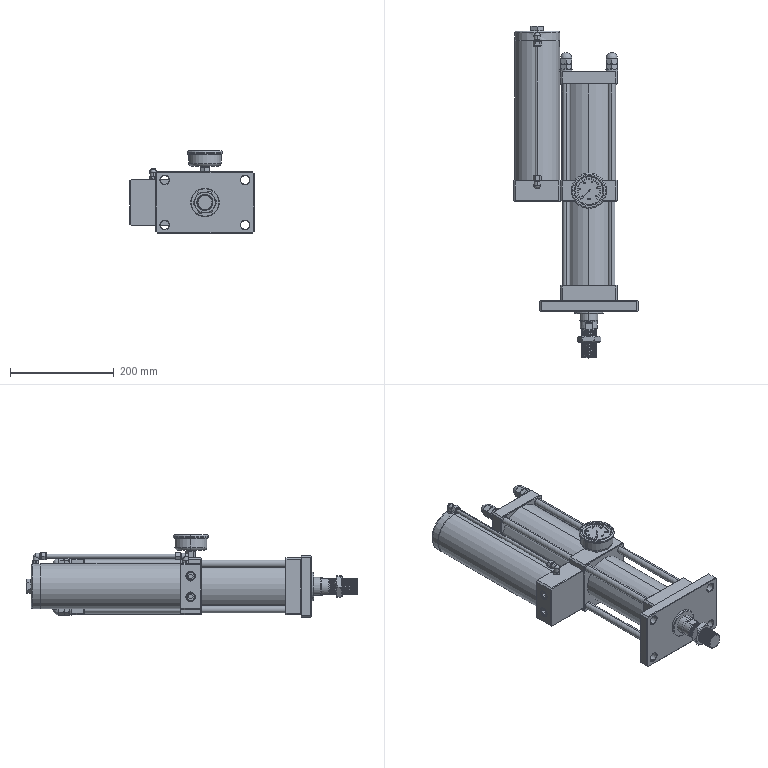Part | STEP file | STA-80-100-10-5T-Xuntuo | 7 solids | 1306 faces | box 240 x 641 x 158.4 mm | volume 3516395 mm3 | plane 640 | cone 269 | cylinder 212 | spline 161 | torus 14 | sphere 10 | commonest cylinder face diameters 30 x70 14 x18 28.5 x14 17 x12 11 x8 12.5 x8